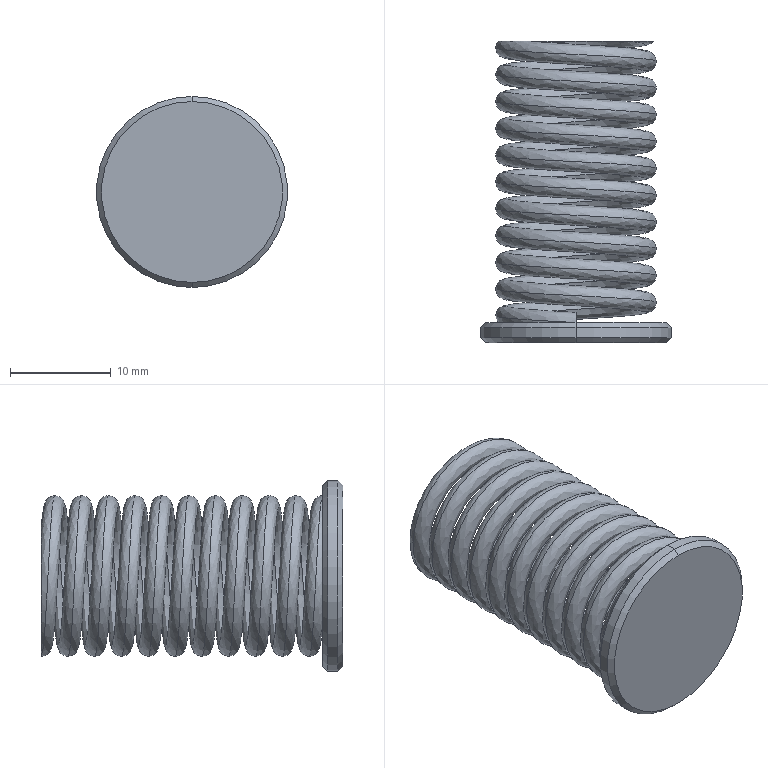Part | STEP file | Medium blue spring TB - TB16-89 | 1 solid | 12 faces | box 19 x 30 x 19 mm | volume 1997 mm3 | cone 4 | plane 4 | cylinder 2 | spline 2 | commonest cylinder face diameters 19 x2